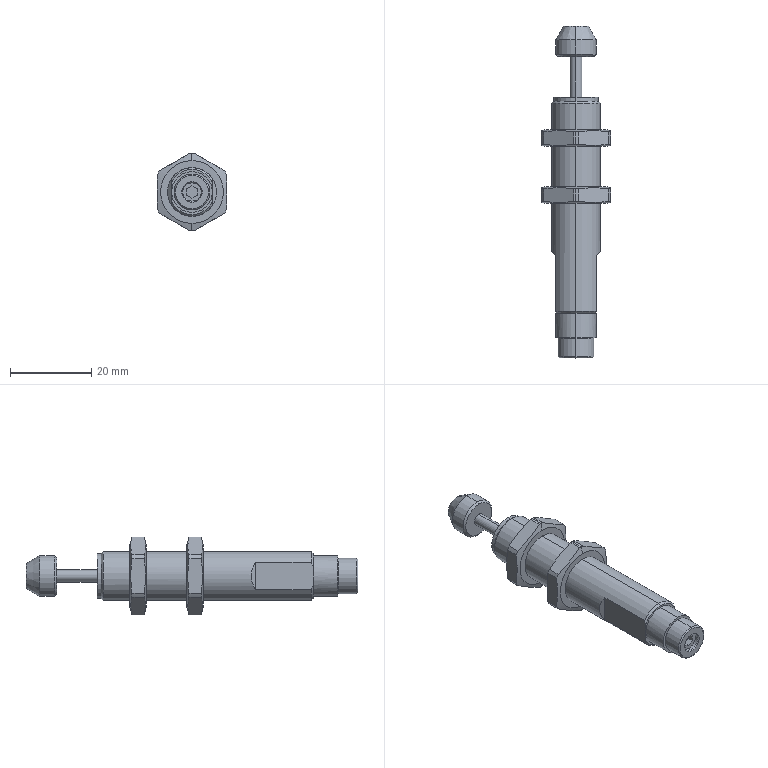Part | STEP file | buffer ACJ1210 | 3 solids | 101 faces | box 17 x 81.5 x 19.048 mm | volume 8306 mm3 | plane 36 | cone 33 | cylinder 32 | commonest cylinder face diameters 19.048 x14 10 x4 11.188 x4 3 x2 4.459 x2 8.8 x2